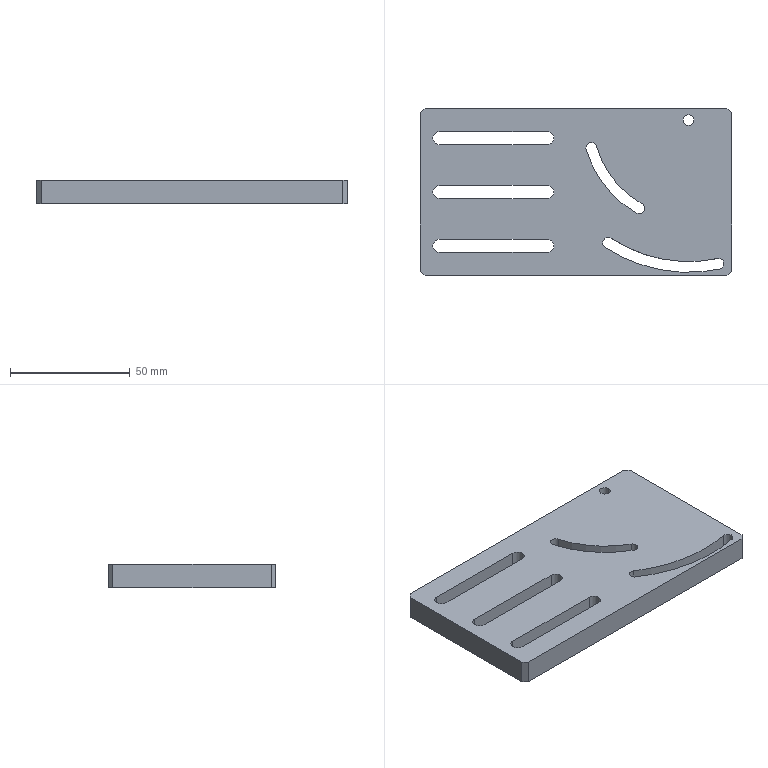CAM job | NX | 3-axis milling, drilling | part box 130 x 70 x 10 mm | stock box 135 x 75 x 12 mm
Tools:
number,name,description,diameter,corner_radius,flute_length,length,flutes
4,D4,平底铣刀-粗,4.0,0.0,25.0,75.0,2
9,D10,平底铣刀-粗,10.0,0.0,35.0,75.0,2
17,D4-J,平底铣刀-精,4.0,0.0,50.0,75.0,2
10,D10-J,平底铣刀-精,10.0,0.0,35.0,75.0,2
1,D80R0.8飞刀,圆鼻刀-粗,80.0,0.8,50.0,75.0,2
1,D80R0.8飞刀-J,圆鼻刀-精,80.0,0.8,50.0,75.0,2
2,D6倒角刀,倒角刀,6.0,0.0,3.0,25.0,2
11,ZT4.5,钻头,4.5,0.0,35.0,50.0,2
Operations:
program,operation,operation_type,tool,method,geometry_group,spindle_rpm,surface_speed,feed_per_tooth,feed_cut,feed_plunge,cut_length_mm,path_length_mm,cut_time_min,machine_time_min
B,底壁铣飞面一刀开粗_COPY,VolumeBased25DMillingOperation,D80R0.8飞刀,分层开粗-切深K-步距G,W-B,5000.0,1256.637,0.3,3000.0,100.0,952.776,1689.884,0.3176,0.3913
B,底壁铣飞面一刀精光_COPY,VolumeBased25DMillingOperation,D80R0.8飞刀-J,侧刃精光-切深K-步距G,W-B,5000.0,1256.637,0.1,1000.0,100.0,237.998,273.998,0.238,0.2416
B,钻倒角_1,Operation,D6倒角刀,METHOD,W-B,8000.0,150.796,0.0625,1000.0,0.0,5.55,51.1,0.0056,0.0101
B,平面去毛刺6X45L_COPY,SurfaceContour,D6倒角刀,爬面_倒角-切深0-步距G,W-B,6500.0,122.519,0.1154,1500.0,100.0,916.575,1358.76,0.6111,0.6553
A,顶面,FaceMilling,D80R0.8飞刀,侧刃精光-切深K-步距G,W-A,4000.0,1005.31,0.125,1000.0,100.0,224.0,260.0,0.224,0.2276
A,外形粗_2,VolumeBased25DMillingOperation,D10,METHOD,W-A,8000.0,251.327,0.3125,5000.0,80.0,9403.381,9451.881,1.881,1.885
A,打点-深0.8,Operation,D6倒角刀,NONE,W-A,8000.0,150.796,0.0312,500.0,90.0,19.8,546.565,0.0396,0.0923
A,通孔-5-6,Operation,ZT4.5,NONE,W-A,3000.0,42.411,0.025,150.0,90.0,157.871,778.01,1.052,1.115
A,通腰槽粗_1,VolumeBased25DMillingOperation,D4,METHOD,W-A,8000.0,100.531,0.1562,2500.0,100.0,19498.576,19879.834,7.799,7.838
A,腰槽精_1,VolumeBased25DMillingOperation,D4-J,METHOD,W-A,6000.0,113.0,0.0667,800.0,100.0,200.464,331.495,0.2506,0.2637
A,腰槽精_2,VolumeBased25DMillingOperation,D4-J,METHOD,W-A,6000.0,113.0,0.0667,800.0,100.0,140.213,211.11,0.1753,0.1824
A,腰槽精_3,VolumeBased25DMillingOperation,D4-J,METHOD,W-A,6000.0,113.0,0.0667,800.0,100.0,581.644,840.368,0.7271,0.7529
A,仅选体,SurfaceContour,D6倒角刀,METHOD,W-A,8000.0,150.796,0.1875,3000.0,100.0,930.242,1317.125,0.3101,0.3488
A,铣倒角_1,PlanarMilling,D6倒角刀,METHOD,W-A,8000.0,150.796,0.0312,500.0,100.0,17.353,58.353,0.0347,0.0388
A,外形半精_2,VolumeBased25DMillingOperation,D10-J,METHOD,W-A,8000.0,251.327,0.0625,1000.0,100.0,431.688,490.688,0.4317,0.4376